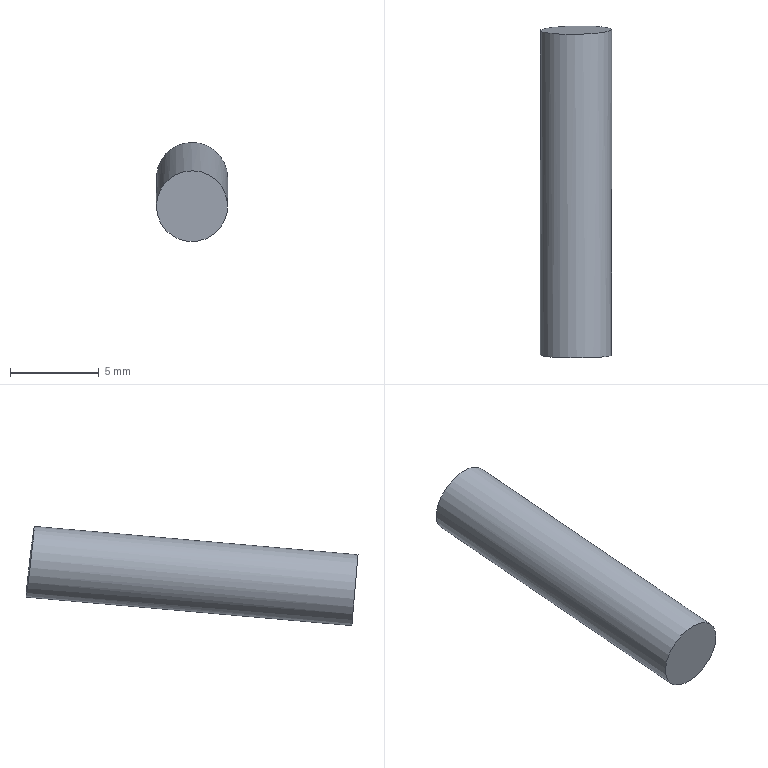Part | NX | features solid 2 | 1 solid | 3 faces | box 4 x 18.66 x 5.576 mm | volume 230.224 mm3 | plane 2 | cylinder 1 | commonest cylinder face diameters 4 x1
STEP:
#1=CARTESIAN_POINT('',(-133.187,40.036,-39.391));
#2=VERTEX_POINT('',#1);
#3=CARTESIAN_POINT('',(-131.187,40.036,-39.391));
#4=DIRECTION('',(0.,0.9962,0.08716));
#5=DIRECTION('',(-1.,0.,0.));
#6=AXIS2_PLACEMENT_3D('',#3,#4,#5);
#7=CIRCLE('',#6,2.);
#8=EDGE_CURVE('',#2,#2,#7,.T.);
#9=ORIENTED_EDGE('',*,*,#8,.F.);
#10=EDGE_LOOP('',(#9));
#11=FACE_BOUND('',#10,.T.);
#12=CARTESIAN_POINT('',(-131.187,40.036,-39.391));
#13=DIRECTION('',(0.,-0.9962,-0.08716));
#14=DIRECTION('',(1.,0.,0.));
#15=AXIS2_PLACEMENT_3D('',#12,#13,#14);
#16=PLANE('',#15);
#17=ADVANCED_FACE('',(#11),#16,.T.);
#18=CARTESIAN_POINT('',(-132.11,58.067,-36.032));
#19=VERTEX_POINT('',#18);
#20=CARTESIAN_POINT('',(-131.187,58.287,-37.794));
#21=DIRECTION('',(-0.01517,0.9931,0.1162));
#22=DIRECTION('',(-0.4611,-0.11,0.8805));
#23=AXIS2_PLACEMENT_3D('',#20,#21,#22);
#24=ELLIPSE('',#23,2.001,2.);
#25=EDGE_CURVE('',#19,#19,#24,.F.);
#26=ORIENTED_EDGE('',*,*,#25,.F.);
#27=EDGE_LOOP('',(#26));
#28=FACE_BOUND('',#27,.T.);
#29=CARTESIAN_POINT('',(-173.425,42.623,90.607));
#30=DIRECTION('',(-0.01517,0.9931,0.1162));
#31=DIRECTION('',(0.05188,0.1168,-0.9918));
#32=AXIS2_PLACEMENT_3D('',#29,#30,#31);
#33=PLANE('',#32);
#34=ADVANCED_FACE('',(#28),#33,.T.);
#35=ORIENTED_EDGE('',*,*,#8,.T.);
#36=EDGE_LOOP('',(#35));
#37=FACE_BOUND('',#36,.T.);
#38=ORIENTED_EDGE('',*,*,#25,.T.);
#39=EDGE_LOOP('',(#38));
#40=FACE_BOUND('',#39,.T.);
#41=CARTESIAN_POINT('',(-131.187,59.96,-37.647));
#42=DIRECTION('',(0.,-0.9962,-0.08716));
#43=DIRECTION('',(1.,0.,0.));
#44=AXIS2_PLACEMENT_3D('',#41,#42,#43);
#45=CYLINDRICAL_SURFACE('',#44,2.);
#46=ADVANCED_FACE('',(#37,#40),#45,.T.);
#47=CLOSED_SHELL('',(#17,#34,#46));
#48=MANIFOLD_SOLID_BREP('',#47);
#49=(LENGTH_UNIT()NAMED_UNIT(*)SI_UNIT(.MILLI.,.METRE.));
#50=UNCERTAINTY_MEASURE_WITH_UNIT(LENGTH_MEASURE(0.00001),#49,'','');
#51=(NAMED_UNIT(*)PLANE_ANGLE_UNIT()SI_UNIT($,.RADIAN.));
#52=(NAMED_UNIT(*)SI_UNIT($,.STERADIAN.)SOLID_ANGLE_UNIT());
#53=(GEOMETRIC_REPRESENTATION_CONTEXT(3)GLOBAL_UNCERTAINTY_ASSIGNED_CONTEXT((#50))GLOBAL_UNIT_ASSIGNED_CONTEXT((#49,#51,#52))REPRESENTATION_CONTEXT('',''));
#54=ADVANCED_BREP_SHAPE_REPRESENTATION('',(#48),#53);